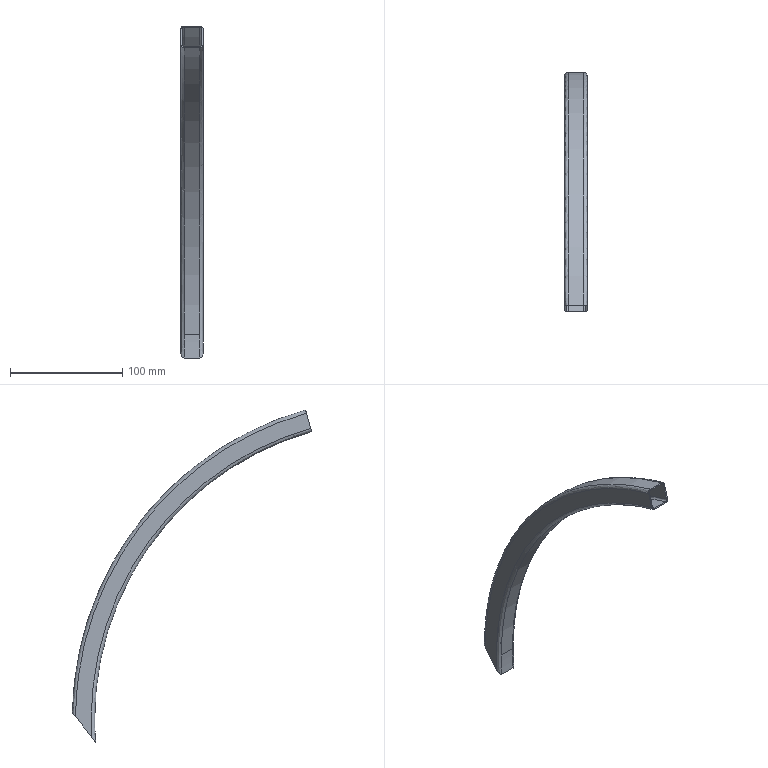Part | SolidWorks | features BaseBody 1 | 1 solid | 20 faces | box 20 x 212.905 x 295.178 mm | volume 31033 mm3 | spline 8 | cylinder 6 | plane 6 | commonest cylinder face diameters 530 x2 532.4 x2 567.6 x1 570 x1